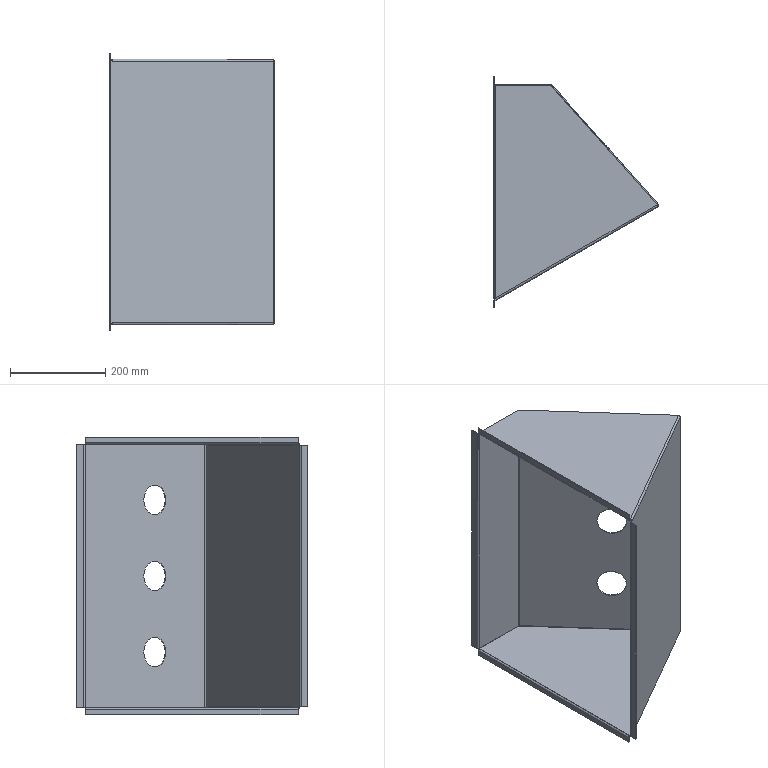Part | STEP file | 750038468 | 1 solid | 64 faces | box 346.594 x 486 x 584 mm | volume 1359967 mm3 | plane 42 | cylinder 22 | commonest cylinder face diameters 4 x8 8 x8 62 x6